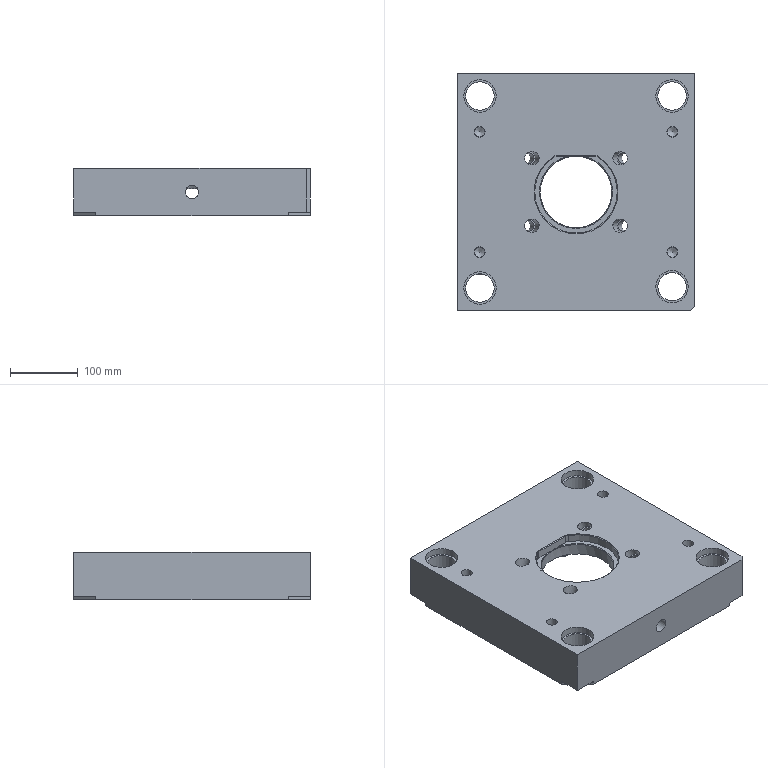Part | NX | features AA 2 | 1 solid | 217 faces | box 350 x 350 x 70 mm | volume 6012843 mm3 | plane 93 | cylinder 74 | spline 32 | cone 14 | sphere 4 | commonest cylinder face diameters 12 x26 10 x12 16 x8 20 x8 15 x4 28 x4